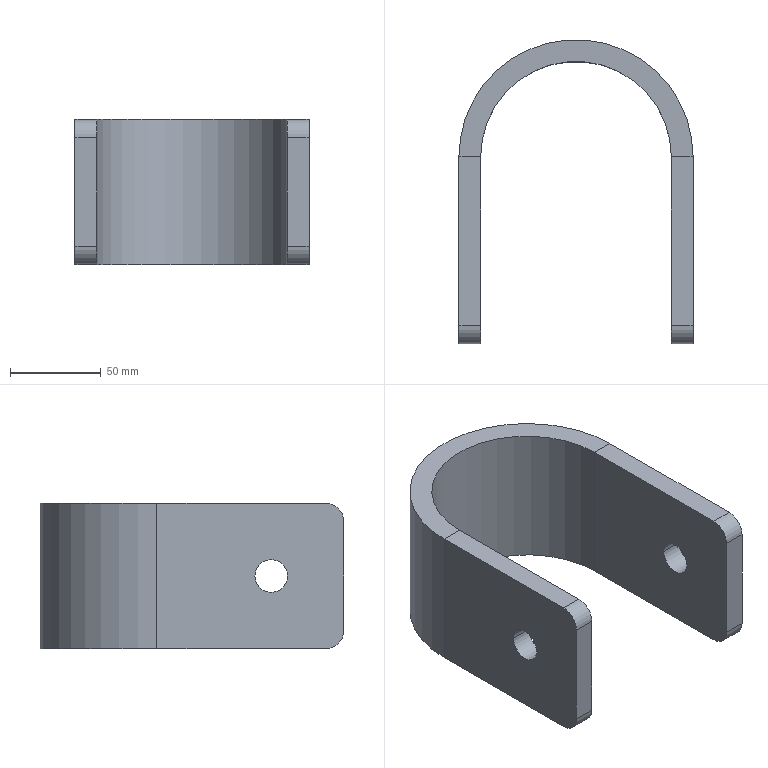Part | STEP file | Coupling rubber strip | 1 solid | 22 faces | box 129 x 167.5 x 80 mm | volume 367054 mm3 | plane 12 | cylinder 10 | commonest cylinder face diameters 18 x4 20 x4 105 x1 129 x1